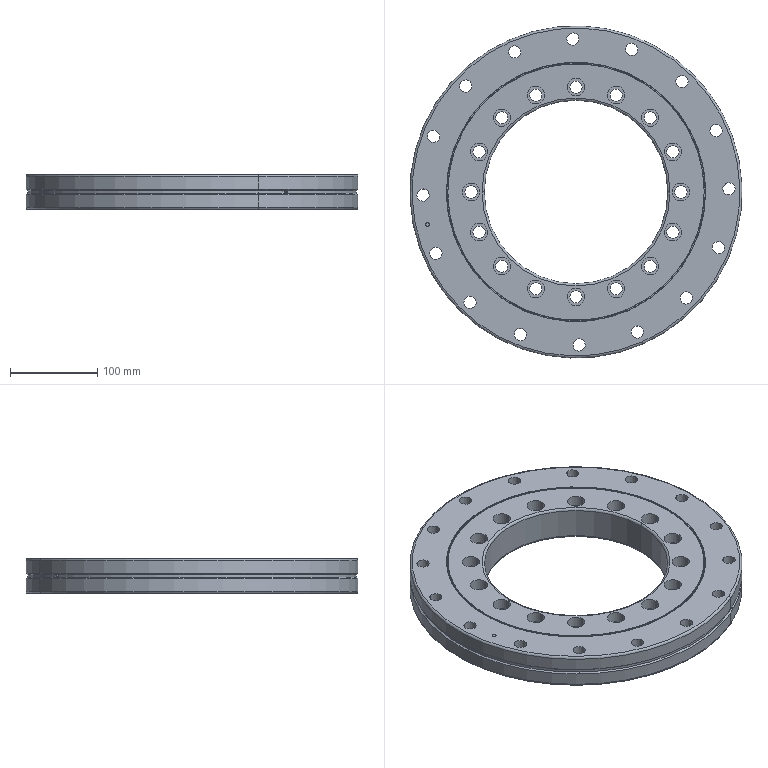Part | SolidWorks | features ReferencePattern 29, CompositeCurve 5, LocalCirPattern 1, MirrorCompFeat 1 | 34 solids | 493 faces | box 380 x 380 x 40 mm | volume 2781012 mm3 | cylinder 227 | torus 138 | plane 108 | cone 20 | commonest cylinder face diameters 14 x64 20 x64 12 x58 293.4 x8 295 x8 296.6 x8